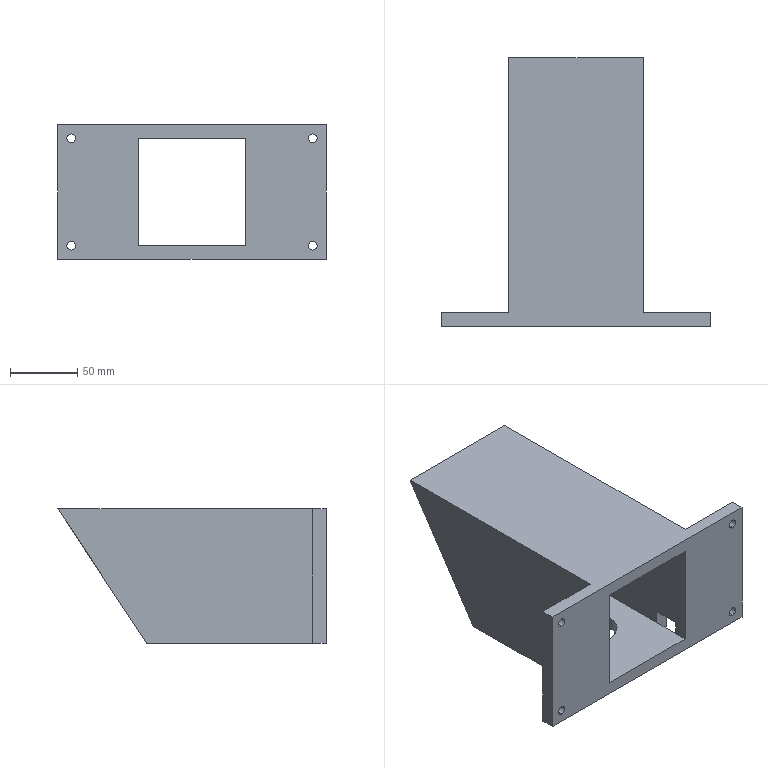Part | SolidWorks | features ICE 4, Extrusion 1, HoleWzd 1 | 1 solid | 35 faces | box 200 x 200 x 100 mm | volume 682330 mm3 | plane 17 | cylinder 10 | cone 8 | commonest cylinder face diameters 6.6 x8 40 x2
STEP:
#1=CARTESIAN_POINT('',(-90.,-93.1,6.7));
#2=VERTEX_POINT('',#1);
#3=CARTESIAN_POINT('',(-90.,-93.1,13.3));
#4=VERTEX_POINT('',#3);
#5=CARTESIAN_POINT('',(-90.,-93.1,10.));
#6=DIRECTION('',(0.,1.,0.));
#7=DIRECTION('',(0.,0.,1.));
#8=AXIS2_PLACEMENT_3D('',#5,#6,#7);
#9=CIRCLE('',#8,3.3);
#10=EDGE_CURVE('',#2,#4,#9,.T.);
#11=ORIENTED_EDGE('',*,*,#10,.F.);
#12=CARTESIAN_POINT('',(-90.,-90.,3.6));
#13=VERTEX_POINT('',#12);
#14=CARTESIAN_POINT('',(-90.,-90.,3.6));
#15=DIRECTION('',(0.,0.7071,-0.7071));
#16=VECTOR('',#15,1000.);
#17=LINE('',#14,#16);
#18=EDGE_CURVE('',#2,#13,#17,.T.);
#19=ORIENTED_EDGE('',*,*,#18,.T.);
#20=CARTESIAN_POINT('',(-90.,-90.,16.4));
#21=VERTEX_POINT('',#20);
#22=CARTESIAN_POINT('',(-90.,-90.,10.));
#23=DIRECTION('',(0.,1.,0.));
#24=DIRECTION('',(0.,0.,1.));
#25=AXIS2_PLACEMENT_3D('',#22,#23,#24);
#26=CIRCLE('',#25,6.4);
#27=EDGE_CURVE('',#13,#21,#26,.T.);
#28=ORIENTED_EDGE('',*,*,#27,.T.);
#29=CARTESIAN_POINT('',(-90.,-90.,16.4));
#30=DIRECTION('',(0.,0.7071,0.7071));
#31=VECTOR('',#30,1000.);
#32=LINE('',#29,#31);
#33=EDGE_CURVE('',#4,#21,#32,.T.);
#34=ORIENTED_EDGE('',*,*,#33,.F.);
#35=EDGE_LOOP('',(#11,#19,#28,#34));
#36=FACE_OUTER_BOUND('',#35,.T.);
#37=CARTESIAN_POINT('',(-90.,-90.,10.));
#38=DIRECTION('',(0.,1.,0.));
#39=DIRECTION('',(0.,0.,1.));
#40=AXIS2_PLACEMENT_3D('',#37,#38,#39);
#41=CONICAL_SURFACE('',#40,6.4,0.7854);
#42=ADVANCED_FACE('',(#36),#41,.F.);
#43=CARTESIAN_POINT('',(-90.,-100.,6.7));
#44=VERTEX_POINT('',#43);
#45=CARTESIAN_POINT('',(-90.,-100.,13.3));
#46=VERTEX_POINT('',#45);
#47=CARTESIAN_POINT('',(-90.,-100.,10.));
#48=DIRECTION('',(0.,1.,0.));
#49=DIRECTION('',(0.,0.,1.));
#50=AXIS2_PLACEMENT_3D('',#47,#48,#49);
#51=CIRCLE('',#50,3.3);
#52=EDGE_CURVE('',#44,#46,#51,.T.);
#53=ORIENTED_EDGE('',*,*,#52,.F.);
#54=CARTESIAN_POINT('',(-90.,-90.,6.7));
#55=DIRECTION('',(0.,1.,0.));
#56=VECTOR('',#55,1000.);
#57=LINE('',#54,#56);
#58=EDGE_CURVE('',#44,#2,#57,.T.);
#59=ORIENTED_EDGE('',*,*,#58,.T.);
#60=ORIENTED_EDGE('',*,*,#10,.T.);
#61=CARTESIAN_POINT('',(-90.,-90.,13.3));
#62=DIRECTION('',(0.,1.,0.));
#63=VECTOR('',#62,1000.);
#64=LINE('',#61,#63);
#65=EDGE_CURVE('',#46,#4,#64,.T.);
#66=ORIENTED_EDGE('',*,*,#65,.F.);
#67=EDGE_LOOP('',(#53,#59,#60,#66));
#68=FACE_OUTER_BOUND('',#67,.T.);
#69=CARTESIAN_POINT('',(-90.,-90.,10.));
#70=DIRECTION('',(0.,1.,0.));
#71=DIRECTION('',(0.,0.,1.));
#72=AXIS2_PLACEMENT_3D('',#69,#70,#71);
#73=CYLINDRICAL_SURFACE('',#72,3.3);
#74=ADVANCED_FACE('',(#68),#73,.F.);
#75=CARTESIAN_POINT('',(-90.,-93.1,86.7));
#76=VERTEX_POINT('',#75);
#77=CARTESIAN_POINT('',(-90.,-93.1,93.3));
#78=VERTEX_POINT('',#77);
#79=CARTESIAN_POINT('',(-90.,-93.1,90.));
#80=DIRECTION('',(0.,1.,0.));
#81=DIRECTION('',(0.,0.,1.));
#82=AXIS2_PLACEMENT_3D('',#79,#80,#81);
#83=CIRCLE('',#82,3.3);
#84=EDGE_CURVE('',#76,#78,#83,.T.);
#85=ORIENTED_EDGE('',*,*,#84,.F.);
#86=CARTESIAN_POINT('',(-90.,-90.,83.6));
#87=VERTEX_POINT('',#86);
#88=CARTESIAN_POINT('',(-90.,-90.,83.6));
#89=DIRECTION('',(0.,0.7071,-0.7071));
#90=VECTOR('',#89,1000.);
#91=LINE('',#88,#90);
#92=EDGE_CURVE('',#76,#87,#91,.T.);
#93=ORIENTED_EDGE('',*,*,#92,.T.);
#94=CARTESIAN_POINT('',(-90.,-90.,96.4));
#95=VERTEX_POINT('',#94);
#96=CARTESIAN_POINT('',(-90.,-90.,90.));
#97=DIRECTION('',(0.,1.,0.));
#98=DIRECTION('',(0.,0.,1.));
#99=AXIS2_PLACEMENT_3D('',#96,#97,#98);
#100=CIRCLE('',#99,6.4);
#101=EDGE_CURVE('',#87,#95,#100,.T.);
#102=ORIENTED_EDGE('',*,*,#101,.T.);
#103=CARTESIAN_POINT('',(-90.,-90.,96.4));
#104=DIRECTION('',(0.,0.7071,0.7071));
#105=VECTOR('',#104,1000.);
#106=LINE('',#103,#105);
#107=EDGE_CURVE('',#78,#95,#106,.T.);
#108=ORIENTED_EDGE('',*,*,#107,.F.);
#109=EDGE_LOOP('',(#85,#93,#102,#108));
#110=FACE_OUTER_BOUND('',#109,.T.);
#111=CARTESIAN_POINT('',(-90.,-90.,90.));
#112=DIRECTION('',(0.,1.,0.));
#113=DIRECTION('',(0.,0.,1.));
#114=AXIS2_PLACEMENT_3D('',#111,#112,#113);
#115=CONICAL_SURFACE('',#114,6.4,0.7854);
#116=ADVANCED_FACE('',(#110),#115,.F.);
#117=CARTESIAN_POINT('',(-90.,-100.,86.7));
#118=VERTEX_POINT('',#117);
#119=CARTESIAN_POINT('',(-90.,-100.,93.3));
#120=VERTEX_POINT('',#119);
#121=CARTESIAN_POINT('',(-90.,-100.,90.));
#122=DIRECTION('',(0.,1.,0.));
#123=DIRECTION('',(0.,0.,1.));
#124=AXIS2_PLACEMENT_3D('',#121,#122,#123);
#125=CIRCLE('',#124,3.3);
#126=EDGE_CURVE('',#118,#120,#125,.T.);
#127=ORIENTED_EDGE('',*,*,#126,.F.);
#128=CARTESIAN_POINT('',(-90.,-90.,86.7));
#129=DIRECTION('',(0.,1.,0.));
#130=VECTOR('',#129,1000.);
#131=LINE('',#128,#130);
#132=EDGE_CURVE('',#118,#76,#131,.T.);
#133=ORIENTED_EDGE('',*,*,#132,.T.);
#134=ORIENTED_EDGE('',*,*,#84,.T.);
#135=CARTESIAN_POINT('',(-90.,-90.,93.3));
#136=DIRECTION('',(0.,1.,0.));
#137=VECTOR('',#136,1000.);
#138=LINE('',#135,#137);
#139=EDGE_CURVE('',#120,#78,#138,.T.);
#140=ORIENTED_EDGE('',*,*,#139,.F.);
#141=EDGE_LOOP('',(#127,#133,#134,#140));
#142=FACE_OUTER_BOUND('',#141,.T.);
#143=CARTESIAN_POINT('',(-90.,-90.,90.));
#144=DIRECTION('',(0.,1.,0.));
#145=DIRECTION('',(0.,0.,1.));
#146=AXIS2_PLACEMENT_3D('',#143,#144,#145);
#147=CYLINDRICAL_SURFACE('',#146,3.3);
#148=ADVANCED_FACE('',(#142),#147,.F.);
#149=CARTESIAN_POINT('',(90.,-93.1,6.7));
#150=VERTEX_POINT('',#149);
#151=CARTESIAN_POINT('',(90.,-93.1,13.3));
#152=VERTEX_POINT('',#151);
#153=CARTESIAN_POINT('',(90.,-93.1,10.));
#154=DIRECTION('',(0.,1.,0.));
#155=DIRECTION('',(0.,0.,1.));
#156=AXIS2_PLACEMENT_3D('',#153,#154,#155);
#157=CIRCLE('',#156,3.3);
#158=EDGE_CURVE('',#150,#152,#157,.T.);
#159=ORIENTED_EDGE('',*,*,#158,.F.);
#160=CARTESIAN_POINT('',(90.,-90.,3.6));
#161=VERTEX_POINT('',#160);
#162=CARTESIAN_POINT('',(90.,-90.,3.6));
#163=DIRECTION('',(0.,0.7071,-0.7071));
#164=VECTOR('',#163,1000.);
#165=LINE('',#162,#164);
#166=EDGE_CURVE('',#150,#161,#165,.T.);
#167=ORIENTED_EDGE('',*,*,#166,.T.);
#168=CARTESIAN_POINT('',(90.,-90.,16.4));
#169=VERTEX_POINT('',#168);
#170=CARTESIAN_POINT('',(90.,-90.,10.));
#171=DIRECTION('',(0.,1.,0.));
#172=DIRECTION('',(0.,0.,1.));
#173=AXIS2_PLACEMENT_3D('',#170,#171,#172);
#174=CIRCLE('',#173,6.4);
#175=EDGE_CURVE('',#161,#169,#174,.T.);
#176=ORIENTED_EDGE('',*,*,#175,.T.);
#177=CARTESIAN_POINT('',(90.,-90.,16.4));
#178=DIRECTION('',(0.,0.7071,0.7071));
#179=VECTOR('',#178,1000.);
#180=LINE('',#177,#179);
#181=EDGE_CURVE('',#152,#169,#180,.T.);
#182=ORIENTED_EDGE('',*,*,#181,.F.);
#183=EDGE_LOOP('',(#159,#167,#176,#182));
#184=FACE_OUTER_BOUND('',#183,.T.);
#185=CARTESIAN_POINT('',(90.,-90.,10.));
#186=DIRECTION('',(0.,1.,0.));
#187=DIRECTION('',(0.,0.,1.));
#188=AXIS2_PLACEMENT_3D('',#185,#186,#187);
#189=CONICAL_SURFACE('',#188,6.4,0.7854);
#190=ADVANCED_FACE('',(#184),#189,.F.);
#191=CARTESIAN_POINT('',(90.,-100.,6.7));
#192=VERTEX_POINT('',#191);
#193=CARTESIAN_POINT('',(90.,-100.,13.3));
#194=VERTEX_POINT('',#193);
#195=CARTESIAN_POINT('',(90.,-100.,10.));
#196=DIRECTION('',(0.,1.,0.));
#197=DIRECTION('',(0.,0.,1.));
#198=AXIS2_PLACEMENT_3D('',#195,#196,#197);
#199=CIRCLE('',#198,3.3);
#200=EDGE_CURVE('',#192,#194,#199,.T.);
#201=ORIENTED_EDGE('',*,*,#200,.F.);
#202=CARTESIAN_POINT('',(90.,-90.,6.7));
#203=DIRECTION('',(0.,1.,0.));
#204=VECTOR('',#203,1000.);
#205=LINE('',#202,#204);
#206=EDGE_CURVE('',#192,#150,#205,.T.);
#207=ORIENTED_EDGE('',*,*,#206,.T.);
#208=ORIENTED_EDGE('',*,*,#158,.T.);
#209=CARTESIAN_POINT('',(90.,-90.,13.3));
#210=DIRECTION('',(0.,1.,0.));
#211=VECTOR('',#210,1000.);
#212=LINE('',#209,#211);
#213=EDGE_CURVE('',#194,#152,#212,.T.);
#214=ORIENTED_EDGE('',*,*,#213,.F.);
#215=EDGE_LOOP('',(#201,#207,#208,#214));
#216=FACE_OUTER_BOUND('',#215,.T.);
#217=CARTESIAN_POINT('',(90.,-90.,10.));
#218=DIRECTION('',(0.,1.,0.));
#219=DIRECTION('',(0.,0.,1.));
#220=AXIS2_PLACEMENT_3D('',#217,#218,#219);
#221=CYLINDRICAL_SURFACE('',#220,3.3);
#222=ADVANCED_FACE('',(#216),#221,.F.);
#223=CARTESIAN_POINT('',(90.,-93.1,86.7));
#224=VERTEX_POINT('',#223);
#225=CARTESIAN_POINT('',(90.,-93.1,93.3));
#226=VERTEX_POINT('',#225);
#227=CARTESIAN_POINT('',(90.,-93.1,90.));
#228=DIRECTION('',(0.,1.,0.));
#229=DIRECTION('',(0.,0.,1.));
#230=AXIS2_PLACEMENT_3D('',#227,#228,#229);
#231=CIRCLE('',#230,3.3);
#232=EDGE_CURVE('',#224,#226,#231,.T.);
#233=ORIENTED_EDGE('',*,*,#232,.F.);
#234=CARTESIAN_POINT('',(90.,-90.,83.6));
#235=VERTEX_POINT('',#234);
#236=CARTESIAN_POINT('',(90.,-90.,83.6));
#237=DIRECTION('',(0.,0.7071,-0.7071));
#238=VECTOR('',#237,1000.);
#239=LINE('',#236,#238);
#240=EDGE_CURVE('',#224,#235,#239,.T.);
#241=ORIENTED_EDGE('',*,*,#240,.T.);
#242=CARTESIAN_POINT('',(90.,-90.,96.4));
#243=VERTEX_POINT('',#242);
#244=CARTESIAN_POINT('',(90.,-90.,90.));
#245=DIRECTION('',(0.,1.,0.));
#246=DIRECTION('',(0.,0.,1.));
#247=AXIS2_PLACEMENT_3D('',#244,#245,#246);
#248=CIRCLE('',#247,6.4);
#249=EDGE_CURVE('',#235,#243,#248,.T.);
#250=ORIENTED_EDGE('',*,*,#249,.T.);
#251=CARTESIAN_POINT('',(90.,-90.,96.4));
#252=DIRECTION('',(0.,0.7071,0.7071));
#253=VECTOR('',#252,1000.);
#254=LINE('',#251,#253);
#255=EDGE_CURVE('',#226,#243,#254,.T.);
#256=ORIENTED_EDGE('',*,*,#255,.F.);
#257=EDGE_LOOP('',(#233,#241,#250,#256));
#258=FACE_OUTER_BOUND('',#257,.T.);
#259=CARTESIAN_POINT('',(90.,-90.,90.));
#260=DIRECTION('',(0.,1.,0.));
#261=DIRECTION('',(0.,0.,1.));
#262=AXIS2_PLACEMENT_3D('',#259,#260,#261);
#263=CONICAL_SURFACE('',#262,6.4,0.7854);
#264=ADVANCED_FACE('',(#258),#263,.F.);
#265=CARTESIAN_POINT('',(90.,-100.,86.7));
#266=VERTEX_POINT('',#265);
#267=CARTESIAN_POINT('',(90.,-100.,93.3));
#268=VERTEX_POINT('',#267);
#269=CARTESIAN_POINT('',(90.,-100.,90.));
#270=DIRECTION('',(0.,1.,0.));
#271=DIRECTION('',(0.,0.,1.));
#272=AXIS2_PLACEMENT_3D('',#269,#270,#271);
#273=CIRCLE('',#272,3.3);
#274=EDGE_CURVE('',#266,#268,#273,.T.);
#275=ORIENTED_EDGE('',*,*,#274,.F.);
#276=CARTESIAN_POINT('',(90.,-90.,86.7));
#277=DIRECTION('',(0.,1.,0.));
#278=VECTOR('',#277,1000.);
#279=LINE('',#276,#278);
#280=EDGE_CURVE('',#266,#224,#279,.T.);
#281=ORIENTED_EDGE('',*,*,#280,.T.);
#282=ORIENTED_EDGE('',*,*,#232,.T.);
#283=CARTESIAN_POINT('',(90.,-90.,93.3));
#284=DIRECTION('',(0.,1.,0.));
#285=VECTOR('',#284,1000.);
#286=LINE('',#283,#285);
#287=EDGE_CURVE('',#268,#226,#286,.T.);
#288=ORIENTED_EDGE('',*,*,#287,.F.);
#289=EDGE_LOOP('',(#275,#281,#282,#288));
#290=FACE_OUTER_BOUND('',#289,.T.);
#291=CARTESIAN_POINT('',(90.,-90.,90.));
#292=DIRECTION('',(0.,1.,0.));
#293=DIRECTION('',(0.,0.,1.));
#294=AXIS2_PLACEMENT_3D('',#291,#292,#293);
#295=CYLINDRICAL_SURFACE('',#294,3.3);
#296=ADVANCED_FACE('',(#290),#295,.F.);
#297=CARTESIAN_POINT('',(20.,-40.,10.));
#298=VERTEX_POINT('',#297);
#299=CARTESIAN_POINT('',(-20.,-40.,10.));
#300=VERTEX_POINT('',#299);
#301=CARTESIAN_POINT('',(0.,-40.,10.));
#302=DIRECTION('',(0.,0.,-1.));
#303=DIRECTION('',(-1.,0.,0.));
#304=AXIS2_PLACEMENT_3D('',#301,#302,#303);
#305=CIRCLE('',#304,20.);
#306=EDGE_CURVE('',#298,#300,#305,.T.);
#307=ORIENTED_EDGE('',*,*,#306,.F.);
#308=CARTESIAN_POINT('',(20.,-40.,0.));
#309=VERTEX_POINT('',#308);
#310=CARTESIAN_POINT('',(20.,-40.,20.));
#311=DIRECTION('',(0.,0.,-1.));
#312=VECTOR('',#311,1000.);
#313=LINE('',#310,#312);
#314=EDGE_CURVE('',#298,#309,#313,.T.);
#315=ORIENTED_EDGE('',*,*,#314,.T.);
#316=CARTESIAN_POINT('',(-20.,-40.,0.));
#317=VERTEX_POINT('',#316);
#318=CARTESIAN_POINT('',(0.,-40.,0.));
#319=DIRECTION('',(0.,0.,-1.));
#320=DIRECTION('',(-1.,0.,0.));
#321=AXIS2_PLACEMENT_3D('',#318,#319,#320);
#322=CIRCLE('',#321,20.);
#323=EDGE_CURVE('',#309,#317,#322,.T.);
#324=ORIENTED_EDGE('',*,*,#323,.T.);
#325=CARTESIAN_POINT('',(-20.,-40.,20.));
#326=DIRECTION('',(0.,0.,-1.));
#327=VECTOR('',#326,1000.);
#328=LINE('',#325,#327);
#329=EDGE_CURVE('',#300,#317,#328,.T.);
#330=ORIENTED_EDGE('',*,*,#329,.F.);
#331=EDGE_LOOP('',(#307,#315,#324,#330));
#332=FACE_OUTER_BOUND('',#331,.T.);
#333=CARTESIAN_POINT('',(0.,-40.,20.));
#334=DIRECTION('',(0.,0.,-1.));
#335=DIRECTION('',(-1.,0.,0.));
#336=AXIS2_PLACEMENT_3D('',#333,#334,#335);
#337=CYLINDRICAL_SURFACE('',#336,20.);
#338=ADVANCED_FACE('',(#332),#337,.F.);
#339=CARTESIAN_POINT('',(50.,-70.,20.));
#340=VERTEX_POINT('',#339);
#341=CARTESIAN_POINT('',(50.,-90.,20.));
#342=VERTEX_POINT('',#341);
#343=CARTESIAN_POINT('',(50.,-90.,20.));
#344=DIRECTION('',(0.,-1.,0.));
#345=VECTOR('',#344,1000.);
#346=LINE('',#343,#345);
#347=EDGE_CURVE('',#340,#342,#346,.T.);
#348=ORIENTED_EDGE('',*,*,#347,.F.);
#349=CARTESIAN_POINT('',(50.,-70.,0.));
#350=VERTEX_POINT('',#349);
#351=CARTESIAN_POINT('',(50.,-70.,0.));
#352=DIRECTION('',(0.,0.,1.));
#353=VECTOR('',#352,1000.);
#354=LINE('',#351,#353);
#355=EDGE_CURVE('',#350,#340,#354,.T.);
#356=ORIENTED_EDGE('',*,*,#355,.F.);
#357=CARTESIAN_POINT('',(50.,33.771,0.));
#358=VERTEX_POINT('',#357);
#359=CARTESIAN_POINT('',(50.,0.,0.));
#360=DIRECTION('',(0.,-1.,0.));
#361=VECTOR('',#360,1000.);
#362=LINE('',#359,#361);
#363=EDGE_CURVE('',#358,#350,#362,.T.);
#364=ORIENTED_EDGE('',*,*,#363,.F.);
#365=CARTESIAN_POINT('',(50.,100.,100.));
#366=VERTEX_POINT('',#365);
#367=CARTESIAN_POINT('',(50.,69.511,53.964));
#368=DIRECTION('',(0.,0.5522,0.8337));
#369=VECTOR('',#368,1000.);
#370=LINE('',#367,#369);
#371=EDGE_CURVE('',#358,#366,#370,.T.);
#372=ORIENTED_EDGE('',*,*,#371,.T.);
#373=CARTESIAN_POINT('',(50.,-90.,100.));
#374=VERTEX_POINT('',#373);
#375=CARTESIAN_POINT('',(50.,0.,100.));
#376=DIRECTION('',(0.,-1.,0.));
#377=VECTOR('',#376,1000.);
#378=LINE('',#375,#377);
#379=EDGE_CURVE('',#366,#374,#378,.T.);
#380=ORIENTED_EDGE('',*,*,#379,.T.);
#381=CARTESIAN_POINT('',(50.,-90.,100.));
#382=DIRECTION('',(0.,0.,-1.));
#383=VECTOR('',#382,1000.);
#384=LINE('',#381,#383);
#385=EDGE_CURVE('',#374,#342,#384,.T.);
#386=ORIENTED_EDGE('',*,*,#385,.T.);
#387=EDGE_LOOP('',(#348,#356,#364,#372,#380,#386));
#388=FACE_OUTER_BOUND('',#387,.T.);
#389=CARTESIAN_POINT('',(50.,0.,100.));
#390=DIRECTION('',(1.,0.,0.));
#391=DIRECTION('',(0.,0.,-1.));
#392=AXIS2_PLACEMENT_3D('',#389,#390,#391);
#393=PLANE('',#392);
#394=ADVANCED_FACE('',(#388),#393,.T.);
#395=CARTESIAN_POINT('',(-50.,33.771,0.));
#396=VERTEX_POINT('',#395);
#397=CARTESIAN_POINT('',(-50.,100.,100.));
#398=VERTEX_POINT('',#397);
#399=CARTESIAN_POINT('',(-50.,69.511,53.964));
#400=DIRECTION('',(0.,0.5522,0.8337));
#401=VECTOR('',#400,1000.);
#402=LINE('',#399,#401);
#403=EDGE_CURVE('',#396,#398,#402,.T.);
#404=ORIENTED_EDGE('',*,*,#403,.F.);
#405=CARTESIAN_POINT('',(-50.,-90.,0.));
#406=VERTEX_POINT('',#405);
#407=CARTESIAN_POINT('',(-50.,0.,0.));
#408=DIRECTION('',(0.,-1.,0.));
#409=VECTOR('',#408,1000.);
#410=LINE('',#407,#409);
#411=EDGE_CURVE('',#396,#406,#410,.T.);
#412=ORIENTED_EDGE('',*,*,#411,.T.);
#413=CARTESIAN_POINT('',(-50.,-90.,100.));
#414=VERTEX_POINT('',#413);
#415=CARTESIAN_POINT('',(-50.,-90.,100.));
#416=DIRECTION('',(0.,0.,-1.));
#417=VECTOR('',#416,1000.);
#418=LINE('',#415,#417);
#419=EDGE_CURVE('',#414,#406,#418,.T.);
#420=ORIENTED_EDGE('',*,*,#419,.F.);
#421=CARTESIAN_POINT('',(-50.,0.,100.));
#422=DIRECTION('',(0.,-1.,0.));
#423=VECTOR('',#422,1000.);
#424=LINE('',#421,#423);
#425=EDGE_CURVE('',#398,#414,#424,.T.);
#426=ORIENTED_EDGE('',*,*,#425,.F.);
#427=EDGE_LOOP('',(#404,#412,#420,#426));
#428=FACE_OUTER_BOUND('',#427,.T.);
#429=CARTESIAN_POINT('',(-50.,0.,100.));
#430=DIRECTION('',(1.,0.,0.));
#431=DIRECTION('',(0.,0.,-1.));
#432=AXIS2_PLACEMENT_3D('',#429,#430,#431);
#433=PLANE('',#432);
#434=ADVANCED_FACE('',(#428),#433,.F.);
#435=CARTESIAN_POINT('',(0.,-40.,0.));
#436=DIRECTION('',(0.,0.,-1.));
#437=DIRECTION('',(-1.,0.,0.));
#438=AXIS2_PLACEMENT_3D('',#435,#436,#437);
#439=CIRCLE('',#438,20.);
#440=EDGE_CURVE('',#317,#309,#439,.T.);
#441=ORIENTED_EDGE('',*,*,#440,.F.);
#442=ORIENTED_EDGE('',*,*,#323,.F.);
#443=EDGE_LOOP('',(#441,#442));
#444=FACE_BOUND('',#443,.T.);
#445=CARTESIAN_POINT('',(40.,-90.,0.));
#446=VERTEX_POINT('',#445);
#447=CARTESIAN_POINT('',(40.,-70.,0.));
#448=VERTEX_POINT('',#447);
#449=CARTESIAN_POINT('',(40.,-90.,0.));
#450=DIRECTION('',(0.,1.,0.));
#451=VECTOR('',#450,1000.);
#452=LINE('',#449,#451);
#453=EDGE_CURVE('',#446,#448,#452,.T.);
#454=ORIENTED_EDGE('',*,*,#453,.F.);
#455=CARTESIAN_POINT('',(100.,-90.,0.));
#456=VERTEX_POINT('',#455);
#457=CARTESIAN_POINT('',(0.,-90.,0.));
#458=DIRECTION('',(1.,0.,0.));
#459=VECTOR('',#458,1000.);
#460=LINE('',#457,#459);
#461=EDGE_CURVE('',#446,#456,#460,.T.);
#462=ORIENTED_EDGE('',*,*,#461,.T.);
#463=CARTESIAN_POINT('',(100.,-100.,0.));
#464=VERTEX_POINT('',#463);
#465=CARTESIAN_POINT('',(100.,0.,0.));
#466=DIRECTION('',(0.,1.,0.));
#467=VECTOR('',#466,1000.);
#468=LINE('',#465,#467);
#469=EDGE_CURVE('',#464,#456,#468,.T.);
#470=ORIENTED_EDGE('',*,*,#469,.F.);
#471=CARTESIAN_POINT('',(-100.,-100.,0.));
#472=VERTEX_POINT('',#471);
#473=CARTESIAN_POINT('',(0.,-100.,0.));
#474=DIRECTION('',(-1.,0.,0.));
#475=VECTOR('',#474,1000.);
#476=LINE('',#473,#475);
#477=EDGE_CURVE('',#464,#472,#476,.T.);
#478=ORIENTED_EDGE('',*,*,#477,.T.);
#479=CARTESIAN_POINT('',(-100.,-90.,0.));
#480=VERTEX_POINT('',#479);
#481=CARTESIAN_POINT('',(-100.,0.,0.));
#482=DIRECTION('',(0.,1.,0.));
#483=VECTOR('',#482,1000.);
#484=LINE('',#481,#483);
#485=EDGE_CURVE('',#472,#480,#484,.T.);
#486=ORIENTED_EDGE('',*,*,#485,.T.);
#487=CARTESIAN_POINT('',(0.,-90.,0.));
#488=DIRECTION('',(-1.,0.,0.));
#489=VECTOR('',#488,1000.);
#490=LINE('',#487,#489);
#491=EDGE_CURVE('',#406,#480,#490,.T.);
#492=ORIENTED_EDGE('',*,*,#491,.F.);
#493=ORIENTED_EDGE('',*,*,#411,.F.);
#494=CARTESIAN_POINT('',(500.,33.771,0.));
#495=DIRECTION('',(-1.,0.,0.));
#496=VECTOR('',#495,1000.);
#497=LINE('',#494,#496);
#498=EDGE_CURVE('',#358,#396,#497,.T.);
#499=ORIENTED_EDGE('',*,*,#498,.F.);
#500=ORIENTED_EDGE('',*,*,#363,.T.);
#501=CARTESIAN_POINT('',(40.,-70.,0.));
#502=DIRECTION('',(1.,0.,0.));
#503=VECTOR('',#502,1000.);
#504=LINE('',#501,#503);
#505=EDGE_CURVE('',#448,#350,#504,.T.);
#506=ORIENTED_EDGE('',*,*,#505,.F.);
#507=EDGE_LOOP('',(#454,#462,#470,#478,#486,#492,#493,#499,#500,#506));
#508=FACE_OUTER_BOUND('',#507,.T.);
#509=CARTESIAN_POINT('',(0.,0.,0.));
#510=DIRECTION('',(0.,0.,1.));
#511=DIRECTION('',(1.,0.,0.));
#512=AXIS2_PLACEMENT_3D('',#509,#510,#511);
#513=PLANE('',#512);
#514=ADVANCED_FACE('',(#444,#508),#513,.F.);
#515=CARTESIAN_POINT('',(-90.,-100.,10.));
#516=DIRECTION('',(0.,1.,0.));
#517=DIRECTION('',(0.,0.,1.));
#518=AXIS2_PLACEMENT_3D('',#515,#516,#517);
#519=CIRCLE('',#518,3.3);
#520=EDGE_CURVE('',#46,#44,#519,.T.);
#521=ORIENTED_EDGE('',*,*,#520,.T.);
#522=ORIENTED_EDGE('',*,*,#52,.T.);
#523=EDGE_LOOP('',(#521,#522));
#524=FACE_BOUND('',#523,.T.);
#525=CARTESIAN_POINT('',(-90.,-100.,90.));
#526=DIRECTION('',(0.,1.,0.));
#527=DIRECTION('',(0.,0.,1.));
#528=AXIS2_PLACEMENT_3D('',#525,#526,#527);
#529=CIRCLE('',#528,3.3);
#530=EDGE_CURVE('',#120,#118,#529,.T.);
#531=ORIENTED_EDGE('',*,*,#530,.T.);
#532=ORIENTED_EDGE('',*,*,#126,.T.);
#533=EDGE_LOOP('',(#531,#532));
#534=FACE_BOUND('',#533,.T.);
#535=CARTESIAN_POINT('',(90.,-100.,10.));
#536=DIRECTION('',(0.,1.,0.));
#537=DIRECTION('',(0.,0.,1.));
#538=AXIS2_PLACEMENT_3D('',#535,#536,#537);
#539=CIRCLE('',#538,3.3);
#540=EDGE_CURVE('',#194,#192,#539,.T.);
#541=ORIENTED_EDGE('',*,*,#540,.T.);
#542=ORIENTED_EDGE('',*,*,#200,.T.);
#543=EDGE_LOOP('',(#541,#542));
#544=FACE_BOUND('',#543,.T.);
#545=CARTESIAN_POINT('',(90.,-100.,90.));
#546=DIRECTION('',(0.,1.,0.));
#547=DIRECTION('',(0.,0.,1.));
#548=AXIS2_PLACEMENT_3D('',#545,#546,#547);
#549=CIRCLE('',#548,3.3);
#550=EDGE_CURVE('',#268,#266,#549,.T.);
#551=ORIENTED_EDGE('',*,*,#550,.T.);
#552=ORIENTED_EDGE('',*,*,#274,.T.);
#553=EDGE_LOOP('',(#551,#552));
#554=FACE_BOUND('',#553,.T.);
#555=CARTESIAN_POINT('',(40.,-100.,90.));
#556=VERTEX_POINT('',#555);
#557=CARTESIAN_POINT('',(40.,-100.,10.));
#558=VERTEX_POINT('',#557);
#559=CARTESIAN_POINT('',(40.,-100.,10.));
#560=DIRECTION('',(0.,0.,-1.));
#561=VECTOR('',#560,1000.);
#562=LINE('',#559,#561);
#563=EDGE_CURVE('',#556,#558,#562,.T.);
#564=ORIENTED_EDGE('',*,*,#563,.T.);
#565=CARTESIAN_POINT('',(-40.,-100.,10.));
#566=VERTEX_POINT('',#565);
#567=CARTESIAN_POINT('',(-40.,-100.,10.));
#568=DIRECTION('',(-1.,0.,0.));
#569=VECTOR('',#568,1000.);
#570=LINE('',#567,#569);
#571=EDGE_CURVE('',#558,#566,#570,.T.);
#572=ORIENTED_EDGE('',*,*,#571,.T.);
#573=CARTESIAN_POINT('',(-40.,-100.,90.));
#574=VERTEX_POINT('',#573);
#575=CARTESIAN_POINT('',(-40.,-100.,10.));
#576=DIRECTION('',(0.,0.,1.));
#577=VECTOR('',#576,1000.);
#578=LINE('',#575,#577);
#579=EDGE_CURVE('',#566,#574,#578,.T.);
#580=ORIENTED_EDGE('',*,*,#579,.T.);
#581=CARTESIAN_POINT('',(-40.,-100.,90.));
#582=DIRECTION('',(1.,0.,0.));
#583=VECTOR('',#582,1000.);
#584=LINE('',#581,#583);
#585=EDGE_CURVE('',#574,#556,#584,.T.);
#586=ORIENTED_EDGE('',*,*,#585,.T.);
#587=EDGE_LOOP('',(#564,#572,#580,#586));
#588=FACE_BOUND('',#587,.T.);
#589=ORIENTED_EDGE('',*,*,#477,.F.);
#590=CARTESIAN_POINT('',(100.,-100.,100.));
#591=VERTEX_POINT('',#590);
#592=CARTESIAN_POINT('',(100.,-100.,100.));
#593=DIRECTION('',(0.,0.,-1.));
#594=VECTOR('',#593,1000.);
#595=LINE('',#592,#594);
#596=EDGE_CURVE('',#591,#464,#595,.T.);
#597=ORIENTED_EDGE('',*,*,#596,.F.);
#598=CARTESIAN_POINT('',(-100.,-100.,100.));
#599=VERTEX_POINT('',#598);
#600=CARTESIAN_POINT('',(0.,-100.,100.));
#601=DIRECTION('',(-1.,0.,0.));
#602=VECTOR('',#601,1000.);
#603=LINE('',#600,#602);
#604=EDGE_CURVE('',#591,#599,#603,.T.);
#605=ORIENTED_EDGE('',*,*,#604,.T.);
#606=CARTESIAN_POINT('',(-100.,-100.,100.));
#607=DIRECTION('',(0.,0.,-1.));
#608=VECTOR('',#607,1000.);
#609=LINE('',#606,#608);
#610=EDGE_CURVE('',#599,#472,#609,.T.);
#611=ORIENTED_EDGE('',*,*,#610,.T.);
#612=EDGE_LOOP('',(#589,#597,#605,#611));
#613=FACE_OUTER_BOUND('',#612,.T.);
#614=CARTESIAN_POINT('',(0.,-100.,100.));
#615=DIRECTION('',(0.,-1.,0.));
#616=DIRECTION('',(0.,0.,-1.));
#617=AXIS2_PLACEMENT_3D('',#614,#615,#616);
#618=PLANE('',#617);
#619=ADVANCED_FACE('',(#524,#534,#544,#554,#588,#613),#618,.T.);
#620=ORIENTED_EDGE('',*,*,#469,.T.);
#621=CARTESIAN_POINT('',(100.,-90.,100.));
#622=VERTEX_POINT('',#621);
#623=CARTESIAN_POINT('',(100.,-90.,100.));
#624=DIRECTION('',(0.,0.,-1.));
#625=VECTOR('',#624,1000.);
#626=LINE('',#623,#625);
#627=EDGE_CURVE('',#622,#456,#626,.T.);
#628=ORIENTED_EDGE('',*,*,#627,.F.);
#629=CARTESIAN_POINT('',(100.,0.,100.));
#630=DIRECTION('',(0.,1.,0.));
#631=VECTOR('',#630,1000.);
#632=LINE('',#629,#631);
#633=EDGE_CURVE('',#591,#622,#632,.T.);
#634=ORIENTED_EDGE('',*,*,#633,.F.);
#635=ORIENTED_EDGE('',*,*,#596,.T.);
#636=EDGE_LOOP('',(#620,#628,#634,#635));
#637=FACE_OUTER_BOUND('',#636,.T.);
#638=CARTESIAN_POINT('',(100.,0.,100.));
#639=DIRECTION('',(-1.,0.,0.));
#640=DIRECTION('',(0.,0.,1.));
#641=AXIS2_PLACEMENT_3D('',#638,#639,#640);
#642=PLANE('',#641);
#643=ADVANCED_FACE('',(#637),#642,.F.);
#644=CARTESIAN_POINT('',(90.,-90.,10.));
#645=DIRECTION('',(0.,1.,0.));
#646=DIRECTION('',(0.,0.,1.));
#647=AXIS2_PLACEMENT_3D('',#644,#645,#646);
#648=CIRCLE('',#647,6.4);
#649=EDGE_CURVE('',#169,#161,#648,.T.);
#650=ORIENTED_EDGE('',*,*,#649,.F.);
#651=ORIENTED_EDGE('',*,*,#175,.F.);
#652=EDGE_LOOP('',(#650,#651));
#653=FACE_BOUND('',#652,.T.);
#654=CARTESIAN_POINT('',(90.,-90.,90.));
#655=DIRECTION('',(0.,1.,0.));
#656=DIRECTION('',(0.,0.,1.));
#657=AXIS2_PLACEMENT_3D('',#654,#655,#656);
#658=CIRCLE('',#657,6.4);
#659=EDGE_CURVE('',#243,#235,#658,.T.);
#660=ORIENTED_EDGE('',*,*,#659,.F.);
#661=ORIENTED_EDGE('',*,*,#249,.F.);
#662=EDGE_LOOP('',(#660,#661));
#663=FACE_BOUND('',#662,.T.);
#664=ORIENTED_EDGE('',*,*,#461,.F.);
#665=CARTESIAN_POINT('',(40.,-90.,10.));
#666=VERTEX_POINT('',#665);
#667=CARTESIAN_POINT('',(40.,-90.,0.));
#668=DIRECTION('',(0.,0.,-1.));
#669=VECTOR('',#668,1000.);
#670=LINE('',#667,#669);
#671=EDGE_CURVE('',#666,#446,#670,.T.);
#672=ORIENTED_EDGE('',*,*,#671,.F.);
#673=CARTESIAN_POINT('',(40.,-90.,20.));
#674=VERTEX_POINT('',#673);
#675=CARTESIAN_POINT('',(40.,-90.,0.));
#676=DIRECTION('',(0.,0.,-1.));
#677=VECTOR('',#676,1000.);
#678=LINE('',#675,#677);
#679=EDGE_CURVE('',#674,#666,#678,.T.);
#680=ORIENTED_EDGE('',*,*,#679,.F.);
#681=CARTESIAN_POINT('',(40.,-90.,20.));
#682=DIRECTION('',(1.,0.,0.));
#683=VECTOR('',#682,1000.);
#684=LINE('',#681,#683);
#685=EDGE_CURVE('',#674,#342,#684,.T.);
#686=ORIENTED_EDGE('',*,*,#685,.T.);
#687=ORIENTED_EDGE('',*,*,#385,.F.);
#688=CARTESIAN_POINT('',(0.,-90.,100.));
#689=DIRECTION('',(1.,0.,0.));
#690=VECTOR('',#689,1000.);
#691=LINE('',#688,#690);
#692=EDGE_CURVE('',#374,#622,#691,.T.);
#693=ORIENTED_EDGE('',*,*,#692,.T.);
#694=ORIENTED_EDGE('',*,*,#627,.T.);
#695=EDGE_LOOP('',(#664,#672,#680,#686,#687,#693,#694));
#696=FACE_OUTER_BOUND('',#695,.T.);
#697=CARTESIAN_POINT('',(0.,-90.,100.));
#698=DIRECTION('',(0.,1.,0.));
#699=DIRECTION('',(0.,0.,1.));
#700=AXIS2_PLACEMENT_3D('',#697,#698,#699);
#701=PLANE('',#700);
#702=ADVANCED_FACE('',(#653,#663,#696),#701,.T.);
#703=CARTESIAN_POINT('',(-90.,-90.,10.));
#704=DIRECTION('',(0.,1.,0.));
#705=DIRECTION('',(0.,0.,1.));
#706=AXIS2_PLACEMENT_3D('',#703,#704,#705);
#707=CIRCLE('',#706,6.4);
#708=EDGE_CURVE('',#21,#13,#707,.T.);
#709=ORIENTED_EDGE('',*,*,#708,.F.);
#710=ORIENTED_EDGE('',*,*,#27,.F.);
#711=EDGE_LOOP('',(#709,#710));
#712=FACE_BOUND('',#711,.T.);
#713=CARTESIAN_POINT('',(-90.,-90.,90.));
#714=DIRECTION('',(0.,1.,0.));
#715=DIRECTION('',(0.,0.,1.));
#716=AXIS2_PLACEMENT_3D('',#713,#714,#715);
#717=CIRCLE('',#716,6.4);
#718=EDGE_CURVE('',#95,#87,#717,.T.);
#719=ORIENTED_EDGE('',*,*,#718,.F.);
#720=ORIENTED_EDGE('',*,*,#101,.F.);
#721=EDGE_LOOP('',(#719,#720));
#722=FACE_BOUND('',#721,.T.);
#723=ORIENTED_EDGE('',*,*,#491,.T.);
#724=CARTESIAN_POINT('',(-100.,-90.,100.));
#725=VERTEX_POINT('',#724);
#726=CARTESIAN_POINT('',(-100.,-90.,100.));
#727=DIRECTION('',(0.,0.,-1.));
#728=VECTOR('',#727,1000.);
#729=LINE('',#726,#728);
#730=EDGE_CURVE('',#725,#480,#729,.T.);
#731=ORIENTED_EDGE('',*,*,#730,.F.);
#732=CARTESIAN_POINT('',(0.,-90.,100.));
#733=DIRECTION('',(-1.,0.,0.));
#734=VECTOR('',#733,1000.);
#735=LINE('',#732,#734);
#736=EDGE_CURVE('',#414,#725,#735,.T.);
#737=ORIENTED_EDGE('',*,*,#736,.F.);
#738=ORIENTED_EDGE('',*,*,#419,.T.);
#739=EDGE_LOOP('',(#723,#731,#737,#738));
#740=FACE_OUTER_BOUND('',#739,.T.);
#741=CARTESIAN_POINT('',(0.,-90.,100.));
#742=DIRECTION('',(0.,-1.,0.));
#743=DIRECTION('',(0.,0.,-1.));
#744=AXIS2_PLACEMENT_3D('',#741,#742,#743);
#745=PLANE('',#744);
#746=ADVANCED_FACE('',(#712,#722,#740),#745,.F.);
#747=ORIENTED_EDGE('',*,*,#485,.F.);
#748=ORIENTED_EDGE('',*,*,#610,.F.);
#749=CARTESIAN_POINT('',(-100.,0.,100.));
#750=DIRECTION('',(0.,1.,0.));
#751=VECTOR('',#750,1000.);
#752=LINE('',#749,#751);
#753=EDGE_CURVE('',#599,#725,#752,.T.);
#754=ORIENTED_EDGE('',*,*,#753,.T.);
#755=ORIENTED_EDGE('',*,*,#730,.T.);
#756=EDGE_LOOP('',(#747,#748,#754,#755));
#757=FACE_OUTER_BOUND('',#756,.T.);
#758=CARTESIAN_POINT('',(-100.,0.,100.));
#759=DIRECTION('',(-1.,0.,0.));
#760=DIRECTION('',(0.,0.,1.));
#761=AXIS2_PLACEMENT_3D('',#758,#759,#760);
#762=PLANE('',#761);
#763=ADVANCED_FACE('',(#757),#762,.T.);
#764=ORIENTED_EDGE('',*,*,#604,.F.);
#765=ORIENTED_EDGE('',*,*,#633,.T.);
#766=ORIENTED_EDGE('',*,*,#692,.F.);
#767=ORIENTED_EDGE('',*,*,#379,.F.);
#768=CARTESIAN_POINT('',(0.,100.,100.));
#769=DIRECTION('',(1.,0.,0.));
#770=VECTOR('',#769,1000.);
#771=LINE('',#768,#770);
#772=EDGE_CURVE('',#398,#366,#771,.T.);
#773=ORIENTED_EDGE('',*,*,#772,.F.);
#774=ORIENTED_EDGE('',*,*,#425,.T.);
#775=ORIENTED_EDGE('',*,*,#736,.T.);
#776=ORIENTED_EDGE('',*,*,#753,.F.);
#777=EDGE_LOOP('',(#764,#765,#766,#767,#773,#774,#775,#776));
#778=FACE_OUTER_BOUND('',#777,.T.);
#779=CARTESIAN_POINT('',(0.,0.,100.));
#780=DIRECTION('',(0.,0.,1.));
#781=DIRECTION('',(1.,0.,0.));
#782=AXIS2_PLACEMENT_3D('',#779,#780,#781);
#783=PLANE('',#782);
#784=ADVANCED_FACE('',(#778),#783,.T.);
#785=CARTESIAN_POINT('',(40.,93.377,90.));
#786=VERTEX_POINT('',#785);
#787=CARTESIAN_POINT('',(40.,40.394,10.));
#788=VERTEX_POINT('',#787);
#789=CARTESIAN_POINT('',(40.,100.,100.));
#790=DIRECTION('',(0.,-0.5522,-0.8337));
#791=VECTOR('',#790,1000.);
#792=LINE('',#789,#791);
#793=EDGE_CURVE('',#786,#788,#792,.T.);
#794=ORIENTED_EDGE('',*,*,#793,.F.);
#795=CARTESIAN_POINT('',(-40.,93.377,90.));
#796=VERTEX_POINT('',#795);
#797=CARTESIAN_POINT('',(500.,93.377,90.));
#798=DIRECTION('',(1.,0.,0.));
#799=VECTOR('',#798,1000.);
#800=LINE('',#797,#799);
#801=EDGE_CURVE('',#796,#786,#800,.T.);
#802=ORIENTED_EDGE('',*,*,#801,.F.);
#803=CARTESIAN_POINT('',(-40.,40.394,10.));
#804=VERTEX_POINT('',#803);
#805=CARTESIAN_POINT('',(-40.,100.,100.));
#806=DIRECTION('',(0.,0.5522,0.8337));
#807=VECTOR('',#806,1000.);
#808=LINE('',#805,#807);
#809=EDGE_CURVE('',#804,#796,#808,.T.);
#810=ORIENTED_EDGE('',*,*,#809,.F.);
#811=CARTESIAN_POINT('',(500.,40.394,10.));
#812=DIRECTION('',(-1.,0.,0.));
#813=VECTOR('',#812,1000.);
#814=LINE('',#811,#813);
#815=EDGE_CURVE('',#788,#804,#814,.T.);
#816=ORIENTED_EDGE('',*,*,#815,.F.);
#817=EDGE_LOOP('',(#794,#802,#810,#816));
#818=FACE_BOUND('',#817,.T.);
#819=ORIENTED_EDGE('',*,*,#371,.F.);
#820=ORIENTED_EDGE('',*,*,#498,.T.);
#821=ORIENTED_EDGE('',*,*,#403,.T.);
#822=ORIENTED_EDGE('',*,*,#772,.T.);
#823=EDGE_LOOP('',(#819,#820,#821,#822));
#824=FACE_OUTER_BOUND('',#823,.T.);
#825=CARTESIAN_POINT('',(500.,100.,100.));
#826=DIRECTION('',(0.,0.8337,-0.5522));
#827=DIRECTION('',(0.,0.5522,0.8337));
#828=AXIS2_PLACEMENT_3D('',#825,#826,#827);
#829=PLANE('',#828);
#830=ADVANCED_FACE('',(#818,#824),#829,.T.);
#831=CARTESIAN_POINT('',(40.,-70.,20.));
#832=VERTEX_POINT('',#831);
#833=CARTESIAN_POINT('',(40.,-90.,20.));
#834=DIRECTION('',(0.,-1.,0.));
#835=VECTOR('',#834,1000.);
#836=LINE('',#833,#835);
#837=EDGE_CURVE('',#832,#674,#836,.T.);
#838=ORIENTED_EDGE('',*,*,#837,.T.);
#839=ORIENTED_EDGE('',*,*,#679,.T.);
#840=CARTESIAN_POINT('',(40.,-100.,10.));
#841=DIRECTION('',(0.,1.,0.));
#842=VECTOR('',#841,1000.);
#843=LINE('',#840,#842);
#844=EDGE_CURVE('',#558,#666,#843,.T.);
#845=ORIENTED_EDGE('',*,*,#844,.F.);
#846=ORIENTED_EDGE('',*,*,#563,.F.);
#847=CARTESIAN_POINT('',(40.,-100.,90.));
#848=DIRECTION('',(0.,1.,0.));
#849=VECTOR('',#848,1000.);
#850=LINE('',#847,#849);
#851=EDGE_CURVE('',#556,#786,#850,.T.);
#852=ORIENTED_EDGE('',*,*,#851,.T.);
#853=ORIENTED_EDGE('',*,*,#793,.T.);
#854=CARTESIAN_POINT('',(40.,-70.,10.));
#855=VERTEX_POINT('',#854);
#856=CARTESIAN_POINT('',(40.,-100.,10.));
#857=DIRECTION('',(0.,1.,0.));
#858=VECTOR('',#857,1000.);
#859=LINE('',#856,#858);
#860=EDGE_CURVE('',#855,#788,#859,.T.);
#861=ORIENTED_EDGE('',*,*,#860,.F.);
#862=CARTESIAN_POINT('',(40.,-70.,0.));
#863=DIRECTION('',(0.,0.,1.));
#864=VECTOR('',#863,1000.);
#865=LINE('',#862,#864);
#866=EDGE_CURVE('',#855,#832,#865,.T.);
#867=ORIENTED_EDGE('',*,*,#866,.T.);
#868=EDGE_LOOP('',(#838,#839,#845,#846,#852,#853,#861,#867));
#869=FACE_OUTER_BOUND('',#868,.T.);
#870=CARTESIAN_POINT('',(40.,-100.,10.));
#871=DIRECTION('',(1.,0.,0.));
#872=DIRECTION('',(0.,0.,-1.));
#873=AXIS2_PLACEMENT_3D('',#870,#871,#872);
#874=PLANE('',#873);
#875=ADVANCED_FACE('',(#869),#874,.F.);
#876=ORIENTED_EDGE('',*,*,#801,.T.);
#877=ORIENTED_EDGE('',*,*,#851,.F.);
#878=ORIENTED_EDGE('',*,*,#585,.F.);
#879=CARTESIAN_POINT('',(-40.,-100.,90.));
#880=DIRECTION('',(0.,1.,0.));
#881=VECTOR('',#880,1000.);
#882=LINE('',#879,#881);
#883=EDGE_CURVE('',#574,#796,#882,.T.);
#884=ORIENTED_EDGE('',*,*,#883,.T.);
#885=EDGE_LOOP('',(#876,#877,#878,#884));
#886=FACE_OUTER_BOUND('',#885,.T.);
#887=CARTESIAN_POINT('',(-40.,-100.,90.));
#888=DIRECTION('',(0.,0.,1.));
#889=DIRECTION('',(1.,0.,0.));
#890=AXIS2_PLACEMENT_3D('',#887,#888,#889);
#891=PLANE('',#890);
#892=ADVANCED_FACE('',(#886),#891,.F.);
#893=ORIENTED_EDGE('',*,*,#809,.T.);
#894=ORIENTED_EDGE('',*,*,#883,.F.);
#895=ORIENTED_EDGE('',*,*,#579,.F.);
#896=CARTESIAN_POINT('',(-40.,-100.,10.));
#897=DIRECTION('',(0.,1.,0.));
#898=VECTOR('',#897,1000.);
#899=LINE('',#896,#898);
#900=EDGE_CURVE('',#566,#804,#899,.T.);
#901=ORIENTED_EDGE('',*,*,#900,.T.);
#902=EDGE_LOOP('',(#893,#894,#895,#901));
#903=FACE_OUTER_BOUND('',#902,.T.);
#904=CARTESIAN_POINT('',(-40.,-100.,10.));
#905=DIRECTION('',(-1.,0.,0.));
#906=DIRECTION('',(0.,0.,1.));
#907=AXIS2_PLACEMENT_3D('',#904,#905,#906);
#908=PLANE('',#907);
#909=ADVANCED_FACE('',(#903),#908,.F.);
#910=CARTESIAN_POINT('',(0.,-40.,10.));
#911=DIRECTION('',(0.,0.,-1.));
#912=DIRECTION('',(-1.,0.,0.));
#913=AXIS2_PLACEMENT_3D('',#910,#911,#912);
#914=CIRCLE('',#913,20.);
#915=EDGE_CURVE('',#300,#298,#914,.T.);
#916=ORIENTED_EDGE('',*,*,#915,.T.);
#917=ORIENTED_EDGE('',*,*,#306,.T.);
#918=EDGE_LOOP('',(#916,#917));
#919=FACE_BOUND('',#918,.T.);
#920=ORIENTED_EDGE('',*,*,#815,.T.);
#921=ORIENTED_EDGE('',*,*,#900,.F.);
#922=ORIENTED_EDGE('',*,*,#571,.F.);
#923=ORIENTED_EDGE('',*,*,#844,.T.);
#924=CARTESIAN_POINT('',(40.,-100.,10.));
#925=DIRECTION('',(0.,1.,0.));
#926=VECTOR('',#925,1000.);
#927=LINE('',#924,#926);
#928=EDGE_CURVE('',#666,#855,#927,.T.);
#929=ORIENTED_EDGE('',*,*,#928,.T.);
#930=ORIENTED_EDGE('',*,*,#860,.T.);
#931=EDGE_LOOP('',(#920,#921,#922,#923,#929,#930));
#932=FACE_OUTER_BOUND('',#931,.T.);
#933=CARTESIAN_POINT('',(-40.,-100.,10.));
#934=DIRECTION('',(0.,0.,-1.));
#935=DIRECTION('',(-1.,0.,0.));
#936=AXIS2_PLACEMENT_3D('',#933,#934,#935);
#937=PLANE('',#936);
#938=ADVANCED_FACE('',(#919,#932),#937,.F.);
#939=ORIENTED_EDGE('',*,*,#314,.F.);
#940=ORIENTED_EDGE('',*,*,#915,.F.);
#941=ORIENTED_EDGE('',*,*,#329,.T.);
#942=ORIENTED_EDGE('',*,*,#440,.T.);
#943=EDGE_LOOP('',(#939,#940,#941,#942));
#944=FACE_OUTER_BOUND('',#943,.T.);
#945=CARTESIAN_POINT('',(0.,-40.,20.));
#946=DIRECTION('',(0.,0.,-1.));
#947=DIRECTION('',(-1.,0.,0.));
#948=AXIS2_PLACEMENT_3D('',#945,#946,#947);
#949=CYLINDRICAL_SURFACE('',#948,20.);
#950=ADVANCED_FACE('',(#944),#949,.F.);
#951=ORIENTED_EDGE('',*,*,#280,.F.);
#952=ORIENTED_EDGE('',*,*,#550,.F.);
#953=ORIENTED_EDGE('',*,*,#287,.T.);
#954=CARTESIAN_POINT('',(90.,-93.1,90.));
#955=DIRECTION('',(0.,1.,0.));
#956=DIRECTION('',(0.,0.,1.));
#957=AXIS2_PLACEMENT_3D('',#954,#955,#956);
#958=CIRCLE('',#957,3.3);
#959=EDGE_CURVE('',#226,#224,#958,.T.);
#960=ORIENTED_EDGE('',*,*,#959,.T.);
#961=EDGE_LOOP('',(#951,#952,#953,#960));
#962=FACE_OUTER_BOUND('',#961,.T.);
#963=CARTESIAN_POINT('',(90.,-90.,90.));
#964=DIRECTION('',(0.,1.,0.));
#965=DIRECTION('',(0.,0.,1.));
#966=AXIS2_PLACEMENT_3D('',#963,#964,#965);
#967=CYLINDRICAL_SURFACE('',#966,3.3);
#968=ADVANCED_FACE('',(#962),#967,.F.);
#969=ORIENTED_EDGE('',*,*,#240,.F.);
#970=ORIENTED_EDGE('',*,*,#959,.F.);
#971=ORIENTED_EDGE('',*,*,#255,.T.);
#972=ORIENTED_EDGE('',*,*,#659,.T.);
#973=EDGE_LOOP('',(#969,#970,#971,#972));
#974=FACE_OUTER_BOUND('',#973,.T.);
#975=CARTESIAN_POINT('',(90.,-90.,90.));
#976=DIRECTION('',(0.,1.,0.));
#977=DIRECTION('',(0.,0.,1.));
#978=AXIS2_PLACEMENT_3D('',#975,#976,#977);
#979=CONICAL_SURFACE('',#978,6.4,0.7854);
#980=ADVANCED_FACE('',(#974),#979,.F.);
#981=ORIENTED_EDGE('',*,*,#206,.F.);
#982=ORIENTED_EDGE('',*,*,#540,.F.);
#983=ORIENTED_EDGE('',*,*,#213,.T.);
#984=CARTESIAN_POINT('',(90.,-93.1,10.));
#985=DIRECTION('',(0.,1.,0.));
#986=DIRECTION('',(0.,0.,1.));
#987=AXIS2_PLACEMENT_3D('',#984,#985,#986);
#988=CIRCLE('',#987,3.3);
#989=EDGE_CURVE('',#152,#150,#988,.T.);
#990=ORIENTED_EDGE('',*,*,#989,.T.);
#991=EDGE_LOOP('',(#981,#982,#983,#990));
#992=FACE_OUTER_BOUND('',#991,.T.);
#993=CARTESIAN_POINT('',(90.,-90.,10.));
#994=DIRECTION('',(0.,1.,0.));
#995=DIRECTION('',(0.,0.,1.));
#996=AXIS2_PLACEMENT_3D('',#993,#994,#995);
#997=CYLINDRICAL_SURFACE('',#996,3.3);
#998=ADVANCED_FACE('',(#992),#997,.F.);
#999=ORIENTED_EDGE('',*,*,#166,.F.);
#1000=ORIENTED_EDGE('',*,*,#989,.F.);
#1001=ORIENTED_EDGE('',*,*,#181,.T.);
#1002=ORIENTED_EDGE('',*,*,#649,.T.);
#1003=EDGE_LOOP('',(#999,#1000,#1001,#1002));
#1004=FACE_OUTER_BOUND('',#1003,.T.);
#1005=CARTESIAN_POINT('',(90.,-90.,10.));
#1006=DIRECTION('',(0.,1.,0.));
#1007=DIRECTION('',(0.,0.,1.));
#1008=AXIS2_PLACEMENT_3D('',#1005,#1006,#1007);
#1009=CONICAL_SURFACE('',#1008,6.4,0.7854);
#1010=ADVANCED_FACE('',(#1004),#1009,.F.);
#1011=ORIENTED_EDGE('',*,*,#132,.F.);
#1012=ORIENTED_EDGE('',*,*,#530,.F.);
#1013=ORIENTED_EDGE('',*,*,#139,.T.);
#1014=CARTESIAN_POINT('',(-90.,-93.1,90.));
#1015=DIRECTION('',(0.,1.,0.));
#1016=DIRECTION('',(0.,0.,1.));
#1017=AXIS2_PLACEMENT_3D('',#1014,#1015,#1016);
#1018=CIRCLE('',#1017,3.3);
#1019=EDGE_CURVE('',#78,#76,#1018,.T.);
#1020=ORIENTED_EDGE('',*,*,#1019,.T.);
#1021=EDGE_LOOP('',(#1011,#1012,#1013,#1020));
#1022=FACE_OUTER_BOUND('',#1021,.T.);
#1023=CARTESIAN_POINT('',(-90.,-90.,90.));
#1024=DIRECTION('',(0.,1.,0.));
#1025=DIRECTION('',(0.,0.,1.));
#1026=AXIS2_PLACEMENT_3D('',#1023,#1024,#1025);
#1027=CYLINDRICAL_SURFACE('',#1026,3.3);
#1028=ADVANCED_FACE('',(#1022),#1027,.F.);
#1029=ORIENTED_EDGE('',*,*,#92,.F.);
#1030=ORIENTED_EDGE('',*,*,#1019,.F.);
#1031=ORIENTED_EDGE('',*,*,#107,.T.);
#1032=ORIENTED_EDGE('',*,*,#718,.T.);
#1033=EDGE_LOOP('',(#1029,#1030,#1031,#1032));
#1034=FACE_OUTER_BOUND('',#1033,.T.);
#1035=CARTESIAN_POINT('',(-90.,-90.,90.));
#1036=DIRECTION('',(0.,1.,0.));
#1037=DIRECTION('',(0.,0.,1.));
#1038=AXIS2_PLACEMENT_3D('',#1035,#1036,#1037);
#1039=CONICAL_SURFACE('',#1038,6.4,0.7854);
#1040=ADVANCED_FACE('',(#1034),#1039,.F.);
#1041=ORIENTED_EDGE('',*,*,#58,.F.);
#1042=ORIENTED_EDGE('',*,*,#520,.F.);
#1043=ORIENTED_EDGE('',*,*,#65,.T.);
#1044=CARTESIAN_POINT('',(-90.,-93.1,10.));
#1045=DIRECTION('',(0.,1.,0.));
#1046=DIRECTION('',(0.,0.,1.));
#1047=AXIS2_PLACEMENT_3D('',#1044,#1045,#1046);
#1048=CIRCLE('',#1047,3.3);
#1049=EDGE_CURVE('',#4,#2,#1048,.T.);
#1050=ORIENTED_EDGE('',*,*,#1049,.T.);
#1051=EDGE_LOOP('',(#1041,#1042,#1043,#1050));
#1052=FACE_OUTER_BOUND('',#1051,.T.);
#1053=CARTESIAN_POINT('',(-90.,-90.,10.));
#1054=DIRECTION('',(0.,1.,0.));
#1055=DIRECTION('',(0.,0.,1.));
#1056=AXIS2_PLACEMENT_3D('',#1053,#1054,#1055);
#1057=CYLINDRICAL_SURFACE('',#1056,3.3);
#1058=ADVANCED_FACE('',(#1052),#1057,.F.);
#1059=ORIENTED_EDGE('',*,*,#18,.F.);
#1060=ORIENTED_EDGE('',*,*,#1049,.F.);
#1061=ORIENTED_EDGE('',*,*,#33,.T.);
#1062=ORIENTED_EDGE('',*,*,#708,.T.);
#1063=EDGE_LOOP('',(#1059,#1060,#1061,#1062));
#1064=FACE_OUTER_BOUND('',#1063,.T.);
#1065=CARTESIAN_POINT('',(-90.,-90.,10.));
#1066=DIRECTION('',(0.,1.,0.));
#1067=DIRECTION('',(0.,0.,1.));
#1068=AXIS2_PLACEMENT_3D('',#1065,#1066,#1067);
#1069=CONICAL_SURFACE('',#1068,6.4,0.7854);
#1070=ADVANCED_FACE('',(#1064),#1069,.F.);
#1071=ORIENTED_EDGE('',*,*,#928,.F.);
#1072=ORIENTED_EDGE('',*,*,#671,.T.);
#1073=ORIENTED_EDGE('',*,*,#453,.T.);
#1074=CARTESIAN_POINT('',(40.,-70.,0.));
#1075=DIRECTION('',(0.,0.,1.));
#1076=VECTOR('',#1075,1000.);
#1077=LINE('',#1074,#1076);
#1078=EDGE_CURVE('',#448,#855,#1077,.T.);
#1079=ORIENTED_EDGE('',*,*,#1078,.T.);
#1080=EDGE_LOOP('',(#1071,#1072,#1073,#1079));
#1081=FACE_OUTER_BOUND('',#1080,.T.);
#1082=CARTESIAN_POINT('',(40.,0.,0.));
#1083=DIRECTION('',(1.,0.,0.));
#1084=DIRECTION('',(0.,0.,-1.));
#1085=AXIS2_PLACEMENT_3D('',#1082,#1083,#1084);
#1086=PLANE('',#1085);
#1087=ADVANCED_FACE('',(#1081),#1086,.T.);
#1088=ORIENTED_EDGE('',*,*,#347,.T.);
#1089=ORIENTED_EDGE('',*,*,#685,.F.);
#1090=ORIENTED_EDGE('',*,*,#837,.F.);
#1091=CARTESIAN_POINT('',(40.,-70.,20.));
#1092=DIRECTION('',(1.,0.,0.));
#1093=VECTOR('',#1092,1000.);
#1094=LINE('',#1091,#1093);
#1095=EDGE_CURVE('',#832,#340,#1094,.T.);
#1096=ORIENTED_EDGE('',*,*,#1095,.T.);
#1097=EDGE_LOOP('',(#1088,#1089,#1090,#1096));
#1098=FACE_OUTER_BOUND('',#1097,.T.);
#1099=CARTESIAN_POINT('',(40.,-90.,20.));
#1100=DIRECTION('',(0.,0.,1.));
#1101=DIRECTION('',(1.,0.,0.));
#1102=AXIS2_PLACEMENT_3D('',#1099,#1100,#1101);
#1103=PLANE('',#1102);
#1104=ADVANCED_FACE('',(#1098),#1103,.F.);
#1105=ORIENTED_EDGE('',*,*,#355,.T.);
#1106=ORIENTED_EDGE('',*,*,#1095,.F.);
#1107=ORIENTED_EDGE('',*,*,#866,.F.);
#1108=ORIENTED_EDGE('',*,*,#1078,.F.);
#1109=ORIENTED_EDGE('',*,*,#505,.T.);
#1110=EDGE_LOOP('',(#1105,#1106,#1107,#1108,#1109));
#1111=FACE_OUTER_BOUND('',#1110,.T.);
#1112=CARTESIAN_POINT('',(40.,-70.,0.));
#1113=DIRECTION('',(0.,1.,0.));
#1114=DIRECTION('',(0.,0.,1.));
#1115=AXIS2_PLACEMENT_3D('',#1112,#1113,#1114);
#1116=PLANE('',#1115);
#1117=ADVANCED_FACE('',(#1111),#1116,.F.);
#1118=CLOSED_SHELL('',(#42,#74,#116,#148,#190,#222,#264,#296,#338,#394,#434,#514,#619,#643,#702,#746,#763,#784,#830,#875,#892,#909,#938,#950,#968,#980,#998,#1010,#1028,#1040,#1058,#1070,#1087,#1104,#1117));
#1119=MANIFOLD_SOLID_BREP('',#1118);
#1120=CARTESIAN_POINT('',(0.,0.,0.));
#1121=DIRECTION('',(0.,0.,1.));
#1122=DIRECTION('',(1.,0.,0.));
#1123=AXIS2_PLACEMENT_3D('',#1120,#1121,#1122);
#1124=(LENGTH_UNIT()NAMED_UNIT(*)SI_UNIT(.MILLI.,.METRE.));
#1125=UNCERTAINTY_MEASURE_WITH_UNIT(LENGTH_MEASURE(0.00001),#1124,'','');
#1126=(NAMED_UNIT(*)PLANE_ANGLE_UNIT()SI_UNIT($,.RADIAN.));
#1127=(NAMED_UNIT(*)SI_UNIT($,.STERADIAN.)SOLID_ANGLE_UNIT());
#1128=(GEOMETRIC_REPRESENTATION_CONTEXT(3)GLOBAL_UNCERTAINTY_ASSIGNED_CONTEXT((#1125))GLOBAL_UNIT_ASSIGNED_CONTEXT((#1124,#1126,#1127))REPRESENTATION_CONTEXT('',''));
#1129=ADVANCED_BREP_SHAPE_REPRESENTATION('',(#1119,#1123),#1128);